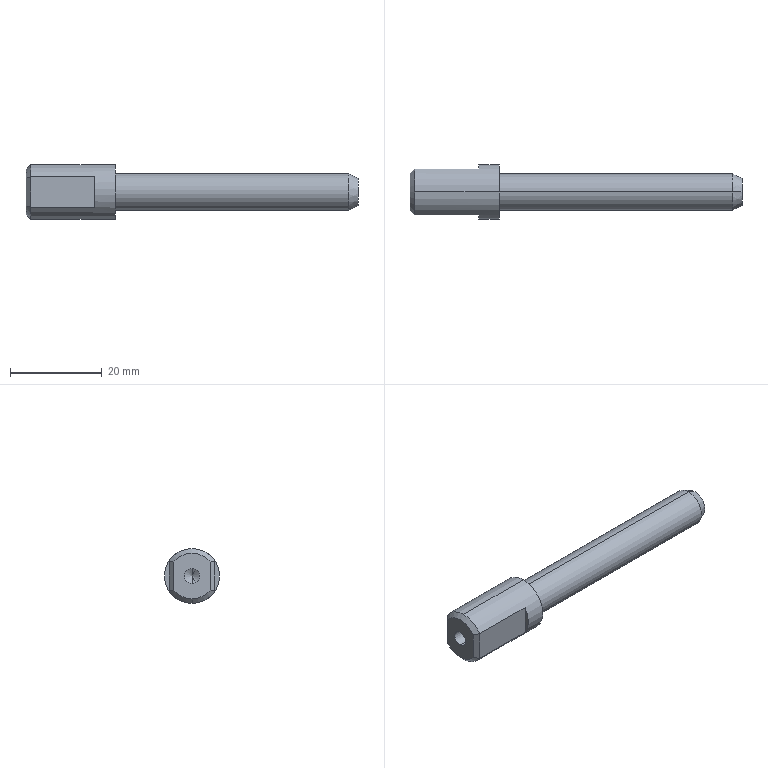Part | SolidWorks | features Chamfer 2, ICE 2, Extrusion 1, HoleWzd 1 | 1 solid | 22 faces | box 72.5 x 12 x 12 mm | volume 4576 mm3 | plane 9 | cone 7 | cylinder 6 | commonest cylinder face diameters 3.3 x2 8 x2 12 x2
STEP:
#1=CARTESIAN_POINT('',(0.,0.,-5.));
#2=VERTEX_POINT('',#1);
#3=CARTESIAN_POINT('',(0.,-4.,-3.));
#4=VERTEX_POINT('',#3);
#5=CARTESIAN_POINT('',(0.,0.,0.));
#6=DIRECTION('',(-1.,0.,0.));
#7=DIRECTION('',(0.,0.,-1.));
#8=AXIS2_PLACEMENT_3D('',#5,#6,#7);
#9=CIRCLE('',#8,5.);
#10=EDGE_CURVE('',#2,#4,#9,.T.);
#11=ORIENTED_EDGE('',*,*,#10,.F.);
#12=CARTESIAN_POINT('',(1.,0.,-6.));
#13=VERTEX_POINT('',#12);
#14=CARTESIAN_POINT('',(1.,0.,-6.));
#15=DIRECTION('',(0.7071,0.,-0.7071));
#16=VECTOR('',#15,1000.);
#17=LINE('',#14,#16);
#18=EDGE_CURVE('',#2,#13,#17,.T.);
#19=ORIENTED_EDGE('',*,*,#18,.T.);
#20=CARTESIAN_POINT('',(1.,-5.,-3.317));
#21=VERTEX_POINT('',#20);
#22=CARTESIAN_POINT('',(1.,0.,0.));
#23=DIRECTION('',(1.,0.,0.));
#24=DIRECTION('',(0.,0.,-1.));
#25=AXIS2_PLACEMENT_3D('',#22,#23,#24);
#26=CIRCLE('',#25,6.);
#27=EDGE_CURVE('',#21,#13,#26,.T.);
#28=ORIENTED_EDGE('',*,*,#27,.F.);
#29=CARTESIAN_POINT('',(0.,-4.,-3.));
#30=CARTESIAN_POINT('',(0.3325,-4.332,-3.111));
#31=CARTESIAN_POINT('',(0.6659,-4.666,-3.216));
#32=CARTESIAN_POINT('',(1.,-5.,-3.317));
#33=B_SPLINE_CURVE_WITH_KNOTS('',3,(#29,#30,#31,#32),.UNSPECIFIED.,.F.,.F.,(4,4),(0.,0.001449),.UNSPECIFIED.);
#34=EDGE_CURVE('',#4,#21,#33,.T.);
#35=ORIENTED_EDGE('',*,*,#34,.F.);
#36=EDGE_LOOP('',(#11,#19,#28,#35));
#37=FACE_OUTER_BOUND('',#36,.T.);
#38=CARTESIAN_POINT('',(1.,0.,0.));
#39=DIRECTION('',(1.,0.,0.));
#40=DIRECTION('',(0.,0.,-1.));
#41=AXIS2_PLACEMENT_3D('',#38,#39,#40);
#42=CONICAL_SURFACE('',#41,6.,0.7854);
#43=ADVANCED_FACE('',(#37),#42,.T.);
#44=CARTESIAN_POINT('',(13.5,0.,-1.65));
#45=VERTEX_POINT('',#44);
#46=CARTESIAN_POINT('',(13.5,0.,1.65));
#47=VERTEX_POINT('',#46);
#48=CARTESIAN_POINT('',(13.5,0.,0.));
#49=DIRECTION('',(-1.,0.,0.));
#50=DIRECTION('',(0.,0.,1.));
#51=AXIS2_PLACEMENT_3D('',#48,#49,#50);
#52=CIRCLE('',#51,1.65);
#53=EDGE_CURVE('',#45,#47,#52,.T.);
#54=ORIENTED_EDGE('',*,*,#53,.F.);
#55=CARTESIAN_POINT('',(0.,0.,-1.65));
#56=VERTEX_POINT('',#55);
#57=CARTESIAN_POINT('',(0.,0.,-1.65));
#58=DIRECTION('',(-1.,0.,0.));
#59=VECTOR('',#58,1000.);
#60=LINE('',#57,#59);
#61=EDGE_CURVE('',#45,#56,#60,.T.);
#62=ORIENTED_EDGE('',*,*,#61,.T.);
#63=CARTESIAN_POINT('',(0.,0.,1.65));
#64=VERTEX_POINT('',#63);
#65=CARTESIAN_POINT('',(0.,0.,0.));
#66=DIRECTION('',(-1.,0.,0.));
#67=DIRECTION('',(0.,0.,1.));
#68=AXIS2_PLACEMENT_3D('',#65,#66,#67);
#69=CIRCLE('',#68,1.65);
#70=EDGE_CURVE('',#56,#64,#69,.T.);
#71=ORIENTED_EDGE('',*,*,#70,.T.);
#72=CARTESIAN_POINT('',(0.,0.,1.65));
#73=DIRECTION('',(-1.,0.,0.));
#74=VECTOR('',#73,1000.);
#75=LINE('',#72,#74);
#76=EDGE_CURVE('',#47,#64,#75,.T.);
#77=ORIENTED_EDGE('',*,*,#76,.F.);
#78=EDGE_LOOP('',(#54,#62,#71,#77));
#79=FACE_OUTER_BOUND('',#78,.T.);
#80=CARTESIAN_POINT('',(0.,0.,0.));
#81=DIRECTION('',(-1.,0.,0.));
#82=DIRECTION('',(0.,0.,1.));
#83=AXIS2_PLACEMENT_3D('',#80,#81,#82);
#84=CYLINDRICAL_SURFACE('',#83,1.65);
#85=ADVANCED_FACE('',(#79),#84,.F.);
#86=CARTESIAN_POINT('',(14.491,0.,0.));
#87=VERTEX_POINT('',#86);
#88=CARTESIAN_POINT('',(13.5,0.,1.65));
#89=DIRECTION('',(-0.515,0.,0.8572));
#90=VECTOR('',#89,1000.);
#91=LINE('',#88,#90);
#92=EDGE_CURVE('',#87,#47,#91,.T.);
#93=ORIENTED_EDGE('',*,*,#92,.F.);
#94=CARTESIAN_POINT('',(13.5,0.,-1.65));
#95=DIRECTION('',(-0.515,0.,-0.8572));
#96=VECTOR('',#95,1000.);
#97=LINE('',#94,#96);
#98=EDGE_CURVE('',#87,#45,#97,.T.);
#99=ORIENTED_EDGE('',*,*,#98,.T.);
#100=ORIENTED_EDGE('',*,*,#53,.T.);
#101=EDGE_LOOP('',(#93,#99,#100));
#102=FACE_OUTER_BOUND('',#101,.T.);
#103=CARTESIAN_POINT('',(13.5,0.,0.));
#104=DIRECTION('',(-1.,0.,0.));
#105=DIRECTION('',(0.,0.,1.));
#106=AXIS2_PLACEMENT_3D('',#103,#104,#105);
#107=CONICAL_SURFACE('',#106,1.65,1.03);
#108=ADVANCED_FACE('',(#102),#107,.F.);
#109=CARTESIAN_POINT('',(72.5,0.,-3.));
#110=VERTEX_POINT('',#109);
#111=CARTESIAN_POINT('',(72.5,0.,3.));
#112=VERTEX_POINT('',#111);
#113=CARTESIAN_POINT('',(72.5,0.,0.));
#114=DIRECTION('',(1.,0.,0.));
#115=DIRECTION('',(0.,0.,-1.));
#116=AXIS2_PLACEMENT_3D('',#113,#114,#115);
#117=CIRCLE('',#116,3.);
#118=EDGE_CURVE('',#110,#112,#117,.T.);
#119=ORIENTED_EDGE('',*,*,#118,.F.);
#120=CARTESIAN_POINT('',(70.5,0.,-4.));
#121=VERTEX_POINT('',#120);
#122=CARTESIAN_POINT('',(72.5,0.,-3.));
#123=DIRECTION('',(-0.8944,0.,-0.4472));
#124=VECTOR('',#123,1000.);
#125=LINE('',#122,#124);
#126=EDGE_CURVE('',#110,#121,#125,.T.);
#127=ORIENTED_EDGE('',*,*,#126,.T.);
#128=CARTESIAN_POINT('',(70.5,0.,4.));
#129=VERTEX_POINT('',#128);
#130=CARTESIAN_POINT('',(70.5,0.,0.));
#131=DIRECTION('',(-1.,0.,0.));
#132=DIRECTION('',(0.,0.,-1.));
#133=AXIS2_PLACEMENT_3D('',#130,#131,#132);
#134=CIRCLE('',#133,4.);
#135=EDGE_CURVE('',#129,#121,#134,.T.);
#136=ORIENTED_EDGE('',*,*,#135,.F.);
#137=CARTESIAN_POINT('',(72.5,0.,3.));
#138=DIRECTION('',(-0.8944,0.,0.4472));
#139=VECTOR('',#138,1000.);
#140=LINE('',#137,#139);
#141=EDGE_CURVE('',#112,#129,#140,.T.);
#142=ORIENTED_EDGE('',*,*,#141,.F.);
#143=EDGE_LOOP('',(#119,#127,#136,#142));
#144=FACE_OUTER_BOUND('',#143,.T.);
#145=CARTESIAN_POINT('',(72.5,0.,0.));
#146=DIRECTION('',(-1.,0.,0.));
#147=DIRECTION('',(0.,0.,1.));
#148=AXIS2_PLACEMENT_3D('',#145,#146,#147);
#149=CONICAL_SURFACE('',#148,3.,0.4636);
#150=ADVANCED_FACE('',(#144),#149,.T.);
#151=ORIENTED_EDGE('',*,*,#135,.T.);
#152=CARTESIAN_POINT('',(19.5,0.,-4.));
#153=VERTEX_POINT('',#152);
#154=CARTESIAN_POINT('',(72.5,0.,-4.));
#155=DIRECTION('',(-1.,0.,0.));
#156=VECTOR('',#155,1000.);
#157=LINE('',#154,#156);
#158=EDGE_CURVE('',#121,#153,#157,.T.);
#159=ORIENTED_EDGE('',*,*,#158,.T.);
#160=CARTESIAN_POINT('',(19.5,0.,4.));
#161=VERTEX_POINT('',#160);
#162=CARTESIAN_POINT('',(19.5,0.,0.));
#163=DIRECTION('',(1.,0.,0.));
#164=DIRECTION('',(0.,0.,-1.));
#165=AXIS2_PLACEMENT_3D('',#162,#163,#164);
#166=CIRCLE('',#165,4.);
#167=EDGE_CURVE('',#153,#161,#166,.T.);
#168=ORIENTED_EDGE('',*,*,#167,.T.);
#169=CARTESIAN_POINT('',(72.5,0.,4.));
#170=DIRECTION('',(-1.,0.,0.));
#171=VECTOR('',#170,1000.);
#172=LINE('',#169,#171);
#173=EDGE_CURVE('',#129,#161,#172,.T.);
#174=ORIENTED_EDGE('',*,*,#173,.F.);
#175=EDGE_LOOP('',(#151,#159,#168,#174));
#176=FACE_OUTER_BOUND('',#175,.T.);
#177=CARTESIAN_POINT('',(72.5,0.,0.));
#178=DIRECTION('',(-1.,0.,0.));
#179=DIRECTION('',(0.,0.,1.));
#180=AXIS2_PLACEMENT_3D('',#177,#178,#179);
#181=CYLINDRICAL_SURFACE('',#180,4.);
#182=ADVANCED_FACE('',(#176),#181,.T.);
#183=CARTESIAN_POINT('',(19.5,0.,-6.));
#184=VERTEX_POINT('',#183);
#185=CARTESIAN_POINT('',(19.5,0.,6.));
#186=VERTEX_POINT('',#185);
#187=CARTESIAN_POINT('',(19.5,0.,0.));
#188=DIRECTION('',(1.,0.,0.));
#189=DIRECTION('',(0.,0.,-1.));
#190=AXIS2_PLACEMENT_3D('',#187,#188,#189);
#191=CIRCLE('',#190,6.);
#192=EDGE_CURVE('',#184,#186,#191,.T.);
#193=ORIENTED_EDGE('',*,*,#192,.F.);
#194=CARTESIAN_POINT('',(19.5,0.,-6.));
#195=DIRECTION('',(-1.,0.,0.));
#196=VECTOR('',#195,1000.);
#197=LINE('',#194,#196);
#198=EDGE_CURVE('',#184,#13,#197,.T.);
#199=ORIENTED_EDGE('',*,*,#198,.T.);
#200=CARTESIAN_POINT('',(1.,5.,-3.317));
#201=VERTEX_POINT('',#200);
#202=CARTESIAN_POINT('',(1.,0.,0.));
#203=DIRECTION('',(1.,0.,0.));
#204=DIRECTION('',(0.,0.,-1.));
#205=AXIS2_PLACEMENT_3D('',#202,#203,#204);
#206=CIRCLE('',#205,6.);
#207=EDGE_CURVE('',#13,#201,#206,.T.);
#208=ORIENTED_EDGE('',*,*,#207,.T.);
#209=CARTESIAN_POINT('',(15.,5.,-3.317));
#210=VERTEX_POINT('',#209);
#211=CARTESIAN_POINT('',(19.5,5.,-3.317));
#212=DIRECTION('',(1.,0.,0.));
#213=VECTOR('',#212,1000.);
#214=LINE('',#211,#213);
#215=EDGE_CURVE('',#201,#210,#214,.T.);
#216=ORIENTED_EDGE('',*,*,#215,.T.);
#217=CARTESIAN_POINT('',(15.,5.,3.317));
#218=VERTEX_POINT('',#217);
#219=CARTESIAN_POINT('',(15.,0.,0.));
#220=DIRECTION('',(1.,0.,0.));
#221=DIRECTION('',(0.,0.,-1.));
#222=AXIS2_PLACEMENT_3D('',#219,#220,#221);
#223=CIRCLE('',#222,6.);
#224=EDGE_CURVE('',#210,#218,#223,.T.);
#225=ORIENTED_EDGE('',*,*,#224,.T.);
#226=CARTESIAN_POINT('',(1.,5.,3.317));
#227=VERTEX_POINT('',#226);
#228=CARTESIAN_POINT('',(19.5,5.,3.317));
#229=DIRECTION('',(-1.,0.,0.));
#230=VECTOR('',#229,1000.);
#231=LINE('',#228,#230);
#232=EDGE_CURVE('',#218,#227,#231,.T.);
#233=ORIENTED_EDGE('',*,*,#232,.T.);
#234=CARTESIAN_POINT('',(1.,0.,6.));
#235=VERTEX_POINT('',#234);
#236=CARTESIAN_POINT('',(1.,0.,0.));
#237=DIRECTION('',(1.,0.,0.));
#238=DIRECTION('',(0.,0.,-1.));
#239=AXIS2_PLACEMENT_3D('',#236,#237,#238);
#240=CIRCLE('',#239,6.);
#241=EDGE_CURVE('',#227,#235,#240,.T.);
#242=ORIENTED_EDGE('',*,*,#241,.T.);
#243=CARTESIAN_POINT('',(19.5,0.,6.));
#244=DIRECTION('',(-1.,0.,0.));
#245=VECTOR('',#244,1000.);
#246=LINE('',#243,#245);
#247=EDGE_CURVE('',#186,#235,#246,.T.);
#248=ORIENTED_EDGE('',*,*,#247,.F.);
#249=EDGE_LOOP('',(#193,#199,#208,#216,#225,#233,#242,#248));
#250=FACE_OUTER_BOUND('',#249,.T.);
#251=CARTESIAN_POINT('',(19.5,0.,0.));
#252=DIRECTION('',(-1.,0.,0.));
#253=DIRECTION('',(0.,0.,1.));
#254=AXIS2_PLACEMENT_3D('',#251,#252,#253);
#255=CYLINDRICAL_SURFACE('',#254,6.);
#256=ADVANCED_FACE('',(#250),#255,.T.);
#257=ORIENTED_EDGE('',*,*,#198,.F.);
#258=CARTESIAN_POINT('',(19.5,0.,0.));
#259=DIRECTION('',(1.,0.,0.));
#260=DIRECTION('',(0.,0.,-1.));
#261=AXIS2_PLACEMENT_3D('',#258,#259,#260);
#262=CIRCLE('',#261,6.);
#263=EDGE_CURVE('',#186,#184,#262,.T.);
#264=ORIENTED_EDGE('',*,*,#263,.F.);
#265=ORIENTED_EDGE('',*,*,#247,.T.);
#266=CARTESIAN_POINT('',(1.,-5.,3.317));
#267=VERTEX_POINT('',#266);
#268=CARTESIAN_POINT('',(1.,0.,0.));
#269=DIRECTION('',(1.,0.,0.));
#270=DIRECTION('',(0.,0.,-1.));
#271=AXIS2_PLACEMENT_3D('',#268,#269,#270);
#272=CIRCLE('',#271,6.);
#273=EDGE_CURVE('',#235,#267,#272,.T.);
#274=ORIENTED_EDGE('',*,*,#273,.T.);
#275=CARTESIAN_POINT('',(15.,-5.,3.317));
#276=VERTEX_POINT('',#275);
#277=CARTESIAN_POINT('',(19.5,-5.,3.317));
#278=DIRECTION('',(1.,0.,0.));
#279=VECTOR('',#278,1000.);
#280=LINE('',#277,#279);
#281=EDGE_CURVE('',#267,#276,#280,.T.);
#282=ORIENTED_EDGE('',*,*,#281,.T.);
#283=CARTESIAN_POINT('',(15.,-5.,-3.317));
#284=VERTEX_POINT('',#283);
#285=CARTESIAN_POINT('',(15.,0.,0.));
#286=DIRECTION('',(1.,0.,0.));
#287=DIRECTION('',(0.,0.,-1.));
#288=AXIS2_PLACEMENT_3D('',#285,#286,#287);
#289=CIRCLE('',#288,6.);
#290=EDGE_CURVE('',#276,#284,#289,.T.);
#291=ORIENTED_EDGE('',*,*,#290,.T.);
#292=CARTESIAN_POINT('',(19.5,-5.,-3.317));
#293=DIRECTION('',(-1.,0.,0.));
#294=VECTOR('',#293,1000.);
#295=LINE('',#292,#294);
#296=EDGE_CURVE('',#284,#21,#295,.T.);
#297=ORIENTED_EDGE('',*,*,#296,.T.);
#298=ORIENTED_EDGE('',*,*,#27,.T.);
#299=EDGE_LOOP('',(#257,#264,#265,#274,#282,#291,#297,#298));
#300=FACE_OUTER_BOUND('',#299,.T.);
#301=CARTESIAN_POINT('',(19.5,0.,0.));
#302=DIRECTION('',(-1.,0.,0.));
#303=DIRECTION('',(0.,0.,1.));
#304=AXIS2_PLACEMENT_3D('',#301,#302,#303);
#305=CYLINDRICAL_SURFACE('',#304,6.);
#306=ADVANCED_FACE('',(#300),#305,.T.);
#307=CARTESIAN_POINT('',(19.5,0.,0.));
#308=DIRECTION('',(1.,0.,0.));
#309=DIRECTION('',(0.,0.,-1.));
#310=AXIS2_PLACEMENT_3D('',#307,#308,#309);
#311=CIRCLE('',#310,4.);
#312=EDGE_CURVE('',#161,#153,#311,.T.);
#313=ORIENTED_EDGE('',*,*,#312,.F.);
#314=ORIENTED_EDGE('',*,*,#167,.F.);
#315=EDGE_LOOP('',(#313,#314));
#316=FACE_BOUND('',#315,.T.);
#317=ORIENTED_EDGE('',*,*,#263,.T.);
#318=ORIENTED_EDGE('',*,*,#192,.T.);
#319=EDGE_LOOP('',(#317,#318));
#320=FACE_OUTER_BOUND('',#319,.T.);
#321=CARTESIAN_POINT('',(19.5,0.,0.));
#322=DIRECTION('',(1.,0.,0.));
#323=DIRECTION('',(0.,0.,-1.));
#324=AXIS2_PLACEMENT_3D('',#321,#322,#323);
#325=PLANE('',#324);
#326=ADVANCED_FACE('',(#316,#320),#325,.T.);
#327=CARTESIAN_POINT('',(0.,4.,-3.));
#328=VERTEX_POINT('',#327);
#329=CARTESIAN_POINT('',(0.,0.,0.));
#330=DIRECTION('',(-1.,0.,0.));
#331=DIRECTION('',(0.,0.,-1.));
#332=AXIS2_PLACEMENT_3D('',#329,#330,#331);
#333=CIRCLE('',#332,5.);
#334=EDGE_CURVE('',#328,#2,#333,.T.);
#335=ORIENTED_EDGE('',*,*,#334,.T.);
#336=ORIENTED_EDGE('',*,*,#10,.T.);
#337=CARTESIAN_POINT('',(0.,-4.,3.));
#338=VERTEX_POINT('',#337);
#339=CARTESIAN_POINT('',(0.,-4.,0.));
#340=DIRECTION('',(0.,0.,1.));
#341=VECTOR('',#340,1000.);
#342=LINE('',#339,#341);
#343=EDGE_CURVE('',#4,#338,#342,.T.);
#344=ORIENTED_EDGE('',*,*,#343,.T.);
#345=CARTESIAN_POINT('',(0.,4.,3.));
#346=VERTEX_POINT('',#345);
#347=CARTESIAN_POINT('',(0.,0.,0.));
#348=DIRECTION('',(-1.,0.,0.));
#349=DIRECTION('',(0.,0.,-1.));
#350=AXIS2_PLACEMENT_3D('',#347,#348,#349);
#351=CIRCLE('',#350,5.);
#352=EDGE_CURVE('',#338,#346,#351,.T.);
#353=ORIENTED_EDGE('',*,*,#352,.T.);
#354=CARTESIAN_POINT('',(0.,4.,0.));
#355=DIRECTION('',(0.,0.,-1.));
#356=VECTOR('',#355,1000.);
#357=LINE('',#354,#356);
#358=EDGE_CURVE('',#346,#328,#357,.T.);
#359=ORIENTED_EDGE('',*,*,#358,.T.);
#360=EDGE_LOOP('',(#335,#336,#344,#353,#359));
#361=FACE_OUTER_BOUND('',#360,.T.);
#362=CARTESIAN_POINT('',(0.,0.,0.));
#363=DIRECTION('',(-1.,0.,0.));
#364=DIRECTION('',(0.,0.,1.));
#365=AXIS2_PLACEMENT_3D('',#362,#363,#364);
#366=CIRCLE('',#365,1.65);
#367=EDGE_CURVE('',#64,#56,#366,.T.);
#368=ORIENTED_EDGE('',*,*,#367,.F.);
#369=ORIENTED_EDGE('',*,*,#70,.F.);
#370=EDGE_LOOP('',(#368,#369));
#371=FACE_BOUND('',#370,.T.);
#372=CARTESIAN_POINT('',(0.,0.,0.));
#373=DIRECTION('',(1.,0.,0.));
#374=DIRECTION('',(0.,0.,-1.));
#375=AXIS2_PLACEMENT_3D('',#372,#373,#374);
#376=PLANE('',#375);
#377=ADVANCED_FACE('',(#361,#371),#376,.F.);
#378=ORIENTED_EDGE('',*,*,#158,.F.);
#379=CARTESIAN_POINT('',(70.5,0.,0.));
#380=DIRECTION('',(-1.,0.,0.));
#381=DIRECTION('',(0.,0.,-1.));
#382=AXIS2_PLACEMENT_3D('',#379,#380,#381);
#383=CIRCLE('',#382,4.);
#384=EDGE_CURVE('',#121,#129,#383,.T.);
#385=ORIENTED_EDGE('',*,*,#384,.T.);
#386=ORIENTED_EDGE('',*,*,#173,.T.);
#387=ORIENTED_EDGE('',*,*,#312,.T.);
#388=EDGE_LOOP('',(#378,#385,#386,#387));
#389=FACE_OUTER_BOUND('',#388,.T.);
#390=CARTESIAN_POINT('',(72.5,0.,0.));
#391=DIRECTION('',(-1.,0.,0.));
#392=DIRECTION('',(0.,0.,1.));
#393=AXIS2_PLACEMENT_3D('',#390,#391,#392);
#394=CYLINDRICAL_SURFACE('',#393,4.);
#395=ADVANCED_FACE('',(#389),#394,.T.);
#396=CARTESIAN_POINT('',(72.5,0.,0.));
#397=DIRECTION('',(1.,0.,0.));
#398=DIRECTION('',(0.,0.,-1.));
#399=AXIS2_PLACEMENT_3D('',#396,#397,#398);
#400=CIRCLE('',#399,3.);
#401=EDGE_CURVE('',#112,#110,#400,.T.);
#402=ORIENTED_EDGE('',*,*,#401,.T.);
#403=ORIENTED_EDGE('',*,*,#118,.T.);
#404=EDGE_LOOP('',(#402,#403));
#405=FACE_OUTER_BOUND('',#404,.T.);
#406=CARTESIAN_POINT('',(72.5,0.,0.));
#407=DIRECTION('',(1.,0.,0.));
#408=DIRECTION('',(0.,0.,-1.));
#409=AXIS2_PLACEMENT_3D('',#406,#407,#408);
#410=PLANE('',#409);
#411=ADVANCED_FACE('',(#405),#410,.T.);
#412=ORIENTED_EDGE('',*,*,#126,.F.);
#413=ORIENTED_EDGE('',*,*,#401,.F.);
#414=ORIENTED_EDGE('',*,*,#141,.T.);
#415=ORIENTED_EDGE('',*,*,#384,.F.);
#416=EDGE_LOOP('',(#412,#413,#414,#415));
#417=FACE_OUTER_BOUND('',#416,.T.);
#418=CARTESIAN_POINT('',(72.5,0.,0.));
#419=DIRECTION('',(-1.,0.,0.));
#420=DIRECTION('',(0.,0.,1.));
#421=AXIS2_PLACEMENT_3D('',#418,#419,#420);
#422=CONICAL_SURFACE('',#421,3.,0.4636);
#423=ADVANCED_FACE('',(#417),#422,.T.);
#424=ORIENTED_EDGE('',*,*,#98,.F.);
#425=ORIENTED_EDGE('',*,*,#92,.T.);
#426=CARTESIAN_POINT('',(13.5,0.,0.));
#427=DIRECTION('',(-1.,0.,0.));
#428=DIRECTION('',(0.,0.,1.));
#429=AXIS2_PLACEMENT_3D('',#426,#427,#428);
#430=CIRCLE('',#429,1.65);
#431=EDGE_CURVE('',#47,#45,#430,.T.);
#432=ORIENTED_EDGE('',*,*,#431,.T.);
#433=EDGE_LOOP('',(#424,#425,#432));
#434=FACE_OUTER_BOUND('',#433,.T.);
#435=CARTESIAN_POINT('',(13.5,0.,0.));
#436=DIRECTION('',(-1.,0.,0.));
#437=DIRECTION('',(0.,0.,1.));
#438=AXIS2_PLACEMENT_3D('',#435,#436,#437);
#439=CONICAL_SURFACE('',#438,1.65,1.03);
#440=ADVANCED_FACE('',(#434),#439,.F.);
#441=ORIENTED_EDGE('',*,*,#61,.F.);
#442=ORIENTED_EDGE('',*,*,#431,.F.);
#443=ORIENTED_EDGE('',*,*,#76,.T.);
#444=ORIENTED_EDGE('',*,*,#367,.T.);
#445=EDGE_LOOP('',(#441,#442,#443,#444));
#446=FACE_OUTER_BOUND('',#445,.T.);
#447=CARTESIAN_POINT('',(0.,0.,0.));
#448=DIRECTION('',(-1.,0.,0.));
#449=DIRECTION('',(0.,0.,1.));
#450=AXIS2_PLACEMENT_3D('',#447,#448,#449);
#451=CYLINDRICAL_SURFACE('',#450,1.65);
#452=ADVANCED_FACE('',(#446),#451,.F.);
#453=CARTESIAN_POINT('',(15.,-5.,6.29));
#454=DIRECTION('',(0.,0.,-1.));
#455=VECTOR('',#454,1000.);
#456=LINE('',#453,#455);
#457=EDGE_CURVE('',#276,#284,#456,.T.);
#458=ORIENTED_EDGE('',*,*,#457,.T.);
#459=ORIENTED_EDGE('',*,*,#290,.F.);
#460=EDGE_LOOP('',(#458,#459));
#461=FACE_OUTER_BOUND('',#460,.T.);
#462=CARTESIAN_POINT('',(15.,0.,0.));
#463=DIRECTION('',(1.,0.,0.));
#464=DIRECTION('',(0.,0.,-1.));
#465=AXIS2_PLACEMENT_3D('',#462,#463,#464);
#466=PLANE('',#465);
#467=ADVANCED_FACE('',(#461),#466,.F.);
#468=ORIENTED_EDGE('',*,*,#281,.F.);
#469=CARTESIAN_POINT('',(1.,-5.,6.29));
#470=DIRECTION('',(0.,0.,-1.));
#471=VECTOR('',#470,1000.);
#472=LINE('',#469,#471);
#473=EDGE_CURVE('',#267,#21,#472,.T.);
#474=ORIENTED_EDGE('',*,*,#473,.T.);
#475=ORIENTED_EDGE('',*,*,#296,.F.);
#476=ORIENTED_EDGE('',*,*,#457,.F.);
#477=EDGE_LOOP('',(#468,#474,#475,#476));
#478=FACE_OUTER_BOUND('',#477,.T.);
#479=CARTESIAN_POINT('',(15.,-5.,6.29));
#480=DIRECTION('',(0.,1.,0.));
#481=DIRECTION('',(0.,0.,1.));
#482=AXIS2_PLACEMENT_3D('',#479,#480,#481);
#483=PLANE('',#482);
#484=ADVANCED_FACE('',(#478),#483,.F.);
#485=CARTESIAN_POINT('',(15.,5.,8.323));
#486=DIRECTION('',(0.,0.,1.));
#487=VECTOR('',#486,1000.);
#488=LINE('',#485,#487);
#489=EDGE_CURVE('',#210,#218,#488,.T.);
#490=ORIENTED_EDGE('',*,*,#489,.T.);
#491=ORIENTED_EDGE('',*,*,#224,.F.);
#492=EDGE_LOOP('',(#490,#491));
#493=FACE_OUTER_BOUND('',#492,.T.);
#494=CARTESIAN_POINT('',(15.,0.,0.));
#495=DIRECTION('',(1.,0.,0.));
#496=DIRECTION('',(0.,0.,-1.));
#497=AXIS2_PLACEMENT_3D('',#494,#495,#496);
#498=PLANE('',#497);
#499=ADVANCED_FACE('',(#493),#498,.F.);
#500=ORIENTED_EDGE('',*,*,#215,.F.);
#501=CARTESIAN_POINT('',(1.,5.,8.323));
#502=DIRECTION('',(0.,0.,1.));
#503=VECTOR('',#502,1000.);
#504=LINE('',#501,#503);
#505=EDGE_CURVE('',#201,#227,#504,.T.);
#506=ORIENTED_EDGE('',*,*,#505,.T.);
#507=ORIENTED_EDGE('',*,*,#232,.F.);
#508=ORIENTED_EDGE('',*,*,#489,.F.);
#509=EDGE_LOOP('',(#500,#506,#507,#508));
#510=FACE_OUTER_BOUND('',#509,.T.);
#511=CARTESIAN_POINT('',(15.,5.,8.323));
#512=DIRECTION('',(0.,-1.,0.));
#513=DIRECTION('',(0.,0.,-1.));
#514=AXIS2_PLACEMENT_3D('',#511,#512,#513);
#515=PLANE('',#514);
#516=ADVANCED_FACE('',(#510),#515,.F.);
#517=CARTESIAN_POINT('',(1.,5.,3.317));
#518=CARTESIAN_POINT('',(0.6659,4.666,3.216));
#519=CARTESIAN_POINT('',(0.3325,4.332,3.111));
#520=CARTESIAN_POINT('',(0.,4.,3.));
#521=B_SPLINE_CURVE_WITH_KNOTS('',3,(#517,#518,#519,#520),.UNSPECIFIED.,.F.,.F.,(4,4),(0.,0.001449),.UNSPECIFIED.);
#522=EDGE_CURVE('',#227,#346,#521,.T.);
#523=ORIENTED_EDGE('',*,*,#522,.F.);
#524=ORIENTED_EDGE('',*,*,#505,.F.);
#525=CARTESIAN_POINT('',(0.,4.,-3.));
#526=CARTESIAN_POINT('',(0.3325,4.332,-3.111));
#527=CARTESIAN_POINT('',(0.6659,4.666,-3.216));
#528=CARTESIAN_POINT('',(1.,5.,-3.317));
#529=B_SPLINE_CURVE_WITH_KNOTS('',3,(#525,#526,#527,#528),.UNSPECIFIED.,.F.,.F.,(4,4),(0.,0.001449),.UNSPECIFIED.);
#530=EDGE_CURVE('',#328,#201,#529,.T.);
#531=ORIENTED_EDGE('',*,*,#530,.F.);
#532=ORIENTED_EDGE('',*,*,#358,.F.);
#533=EDGE_LOOP('',(#523,#524,#531,#532));
#534=FACE_OUTER_BOUND('',#533,.T.);
#535=CARTESIAN_POINT('',(0.,4.,0.));
#536=DIRECTION('',(0.7071,-0.7071,0.));
#537=DIRECTION('',(0.,0.,-1.));
#538=AXIS2_PLACEMENT_3D('',#535,#536,#537);
#539=PLANE('',#538);
#540=ADVANCED_FACE('',(#534),#539,.F.);
#541=ORIENTED_EDGE('',*,*,#18,.F.);
#542=ORIENTED_EDGE('',*,*,#334,.F.);
#543=ORIENTED_EDGE('',*,*,#530,.T.);
#544=ORIENTED_EDGE('',*,*,#207,.F.);
#545=EDGE_LOOP('',(#541,#542,#543,#544));
#546=FACE_OUTER_BOUND('',#545,.T.);
#547=CARTESIAN_POINT('',(1.,0.,0.));
#548=DIRECTION('',(1.,0.,0.));
#549=DIRECTION('',(0.,0.,-1.));
#550=AXIS2_PLACEMENT_3D('',#547,#548,#549);
#551=CONICAL_SURFACE('',#550,6.,0.7854);
#552=ADVANCED_FACE('',(#546),#551,.T.);
#553=ORIENTED_EDGE('',*,*,#522,.T.);
#554=ORIENTED_EDGE('',*,*,#352,.F.);
#555=CARTESIAN_POINT('',(1.,-5.,3.317));
#556=CARTESIAN_POINT('',(0.6659,-4.666,3.216));
#557=CARTESIAN_POINT('',(0.3325,-4.332,3.111));
#558=CARTESIAN_POINT('',(0.,-4.,3.));
#559=B_SPLINE_CURVE_WITH_KNOTS('',3,(#555,#556,#557,#558),.UNSPECIFIED.,.F.,.F.,(4,4),(0.,0.001449),.UNSPECIFIED.);
#560=EDGE_CURVE('',#267,#338,#559,.T.);
#561=ORIENTED_EDGE('',*,*,#560,.F.);
#562=ORIENTED_EDGE('',*,*,#273,.F.);
#563=ORIENTED_EDGE('',*,*,#241,.F.);
#564=EDGE_LOOP('',(#553,#554,#561,#562,#563));
#565=FACE_OUTER_BOUND('',#564,.T.);
#566=CARTESIAN_POINT('',(1.,0.,0.));
#567=DIRECTION('',(1.,0.,0.));
#568=DIRECTION('',(0.,0.,-1.));
#569=AXIS2_PLACEMENT_3D('',#566,#567,#568);
#570=CONICAL_SURFACE('',#569,6.,0.7854);
#571=ADVANCED_FACE('',(#565),#570,.T.);
#572=ORIENTED_EDGE('',*,*,#34,.T.);
#573=ORIENTED_EDGE('',*,*,#473,.F.);
#574=ORIENTED_EDGE('',*,*,#560,.T.);
#575=ORIENTED_EDGE('',*,*,#343,.F.);
#576=EDGE_LOOP('',(#572,#573,#574,#575));
#577=FACE_OUTER_BOUND('',#576,.T.);
#578=CARTESIAN_POINT('',(0.,-4.,0.));
#579=DIRECTION('',(0.7071,0.7071,0.));
#580=DIRECTION('',(0.,0.,1.));
#581=AXIS2_PLACEMENT_3D('',#578,#579,#580);
#582=PLANE('',#581);
#583=ADVANCED_FACE('',(#577),#582,.F.);
#584=CLOSED_SHELL('',(#43,#85,#108,#150,#182,#256,#306,#326,#377,#395,#411,#423,#440,#452,#467,#484,#499,#516,#540,#552,#571,#583));
#585=MANIFOLD_SOLID_BREP('',#584);
#586=CARTESIAN_POINT('',(0.,0.,0.));
#587=DIRECTION('',(0.,0.,1.));
#588=DIRECTION('',(1.,0.,0.));
#589=AXIS2_PLACEMENT_3D('',#586,#587,#588);
#590=(LENGTH_UNIT()NAMED_UNIT(*)SI_UNIT(.MILLI.,.METRE.));
#591=UNCERTAINTY_MEASURE_WITH_UNIT(LENGTH_MEASURE(0.00001),#590,'','');
#592=(NAMED_UNIT(*)PLANE_ANGLE_UNIT()SI_UNIT($,.RADIAN.));
#593=(NAMED_UNIT(*)SI_UNIT($,.STERADIAN.)SOLID_ANGLE_UNIT());
#594=(GEOMETRIC_REPRESENTATION_CONTEXT(3)GLOBAL_UNCERTAINTY_ASSIGNED_CONTEXT((#591))GLOBAL_UNIT_ASSIGNED_CONTEXT((#590,#592,#593))REPRESENTATION_CONTEXT('',''));
#595=ADVANCED_BREP_SHAPE_REPRESENTATION('',(#585,#589),#594);